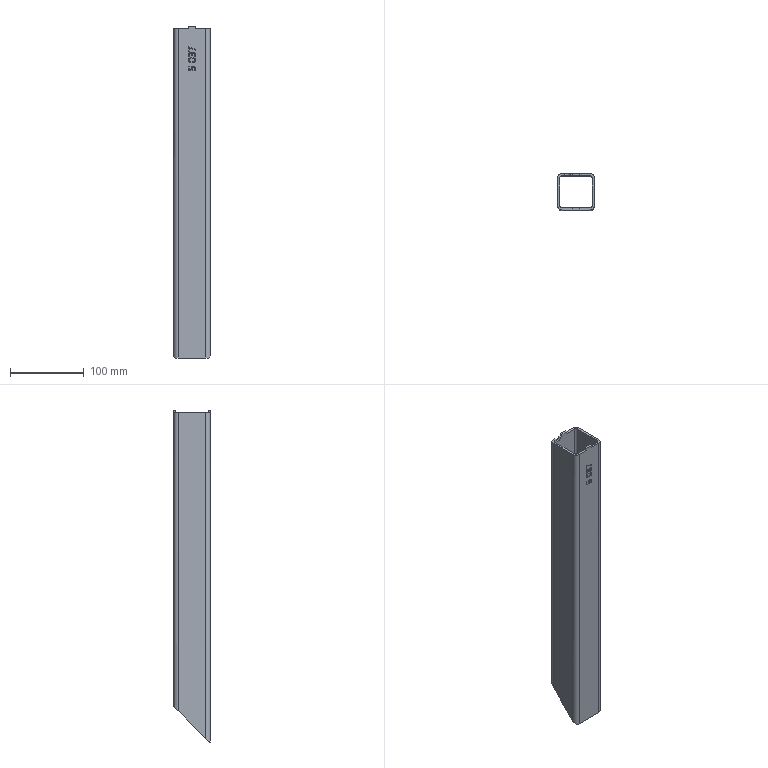Part | SolidWorks | features BaseBody 1 | 1 solid | 84 faces | box 50 x 50 x 451.5 mm | volume 229789 mm3 | plane 46 | spline 29 | cylinder 9 | commonest cylinder face diameters 6 x4 12 x4 8 x1